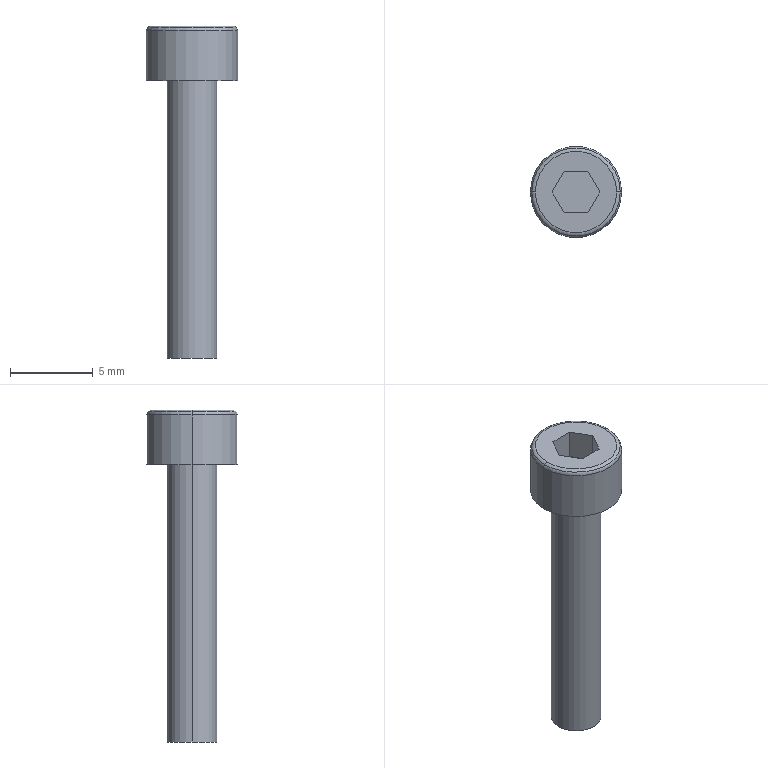Part | Creo | 1 solid | 18 faces | box 5.5 x 5.5 x 20 mm | volume 186.379 mm3 | plane 10 | cylinder 4 | torus 4 | commonest cylinder face diameters 3 x2 5.5 x2
STEP:
#1=CARTESIAN_POINT('',(0.,0.,0.));
#2=DIRECTION('',(0.,0.,1.));
#3=DIRECTION('',(1.,0.,0.));
#4=AXIS2_PLACEMENT_3D('',#1,#2,#3);
#5=CARTESIAN_POINT('',(30.45,156.5,-39.767));
#6=VERTEX_POINT('',#5);
#7=CARTESIAN_POINT('',(33.45,156.5,-39.767));
#8=VERTEX_POINT('',#7);
#9=CARTESIAN_POINT('',(31.95,156.5,-39.767));
#10=DIRECTION('',(0.,0.,-1.));
#11=DIRECTION('',(-1.,0.,0.));
#12=AXIS2_PLACEMENT_3D('',#9,#10,#11);
#13=CIRCLE('',#12,1.5);
#14=EDGE_CURVE('',#6,#8,#13,.T.);
#15=ORIENTED_EDGE('',*,*,#14,.F.);
#16=CARTESIAN_POINT('',(31.95,156.5,-39.767));
#17=DIRECTION('',(0.,0.,-1.));
#18=DIRECTION('',(1.,0.,0.));
#19=AXIS2_PLACEMENT_3D('',#16,#17,#18);
#20=CIRCLE('',#19,1.5);
#21=EDGE_CURVE('',#8,#6,#20,.T.);
#22=ORIENTED_EDGE('',*,*,#21,.F.);
#23=EDGE_LOOP('',(#15,#22));
#24=FACE_OUTER_BOUND('',#23,.F.);
#25=CARTESIAN_POINT('',(31.95,156.5,-39.767));
#26=DIRECTION('',(0.,0.,-1.));
#27=DIRECTION('',(-1.,0.,0.));
#28=AXIS2_PLACEMENT_3D('',#25,#26,#27);
#29=PLANE('',#28);
#30=ADVANCED_FACE('',(#24),#29,.T.);
#31=CARTESIAN_POINT('',(33.45,156.5,-23.067));
#32=VERTEX_POINT('',#31);
#33=CARTESIAN_POINT('',(30.45,156.5,-23.067));
#34=VERTEX_POINT('',#33);
#35=CARTESIAN_POINT('',(31.95,156.5,-23.067));
#36=DIRECTION('',(0.,0.,1.));
#37=DIRECTION('',(1.,0.,0.));
#38=AXIS2_PLACEMENT_3D('',#35,#36,#37);
#39=CIRCLE('',#38,1.5);
#40=EDGE_CURVE('',#32,#34,#39,.T.);
#41=ORIENTED_EDGE('',*,*,#40,.T.);
#42=CARTESIAN_POINT('',(30.45,156.5,-23.067));
#43=DIRECTION('',(0.,0.,-1.));
#44=VECTOR('',#43,16.7);
#45=LINE('',#42,#44);
#46=EDGE_CURVE('',#34,#6,#45,.T.);
#47=ORIENTED_EDGE('',*,*,#46,.T.);
#48=ORIENTED_EDGE('',*,*,#14,.T.);
#49=CARTESIAN_POINT('',(33.45,156.5,-23.067));
#50=DIRECTION('',(0.,0.,-1.));
#51=VECTOR('',#50,16.7);
#52=LINE('',#49,#51);
#53=EDGE_CURVE('',#32,#8,#52,.T.);
#54=ORIENTED_EDGE('',*,*,#53,.F.);
#55=EDGE_LOOP('',(#41,#47,#48,#54));
#56=FACE_OUTER_BOUND('',#55,.F.);
#57=CARTESIAN_POINT('',(31.95,156.5,-19.767));
#58=DIRECTION('',(0.,0.,-1.));
#59=DIRECTION('',(-1.,0.,0.));
#60=AXIS2_PLACEMENT_3D('',#57,#58,#59);
#61=CYLINDRICAL_SURFACE('',#60,1.5);
#62=ADVANCED_FACE('',(#56),#61,.T.);
#63=CARTESIAN_POINT('',(29.2,156.5,-23.067));
#64=VERTEX_POINT('',#63);
#65=CARTESIAN_POINT('',(34.7,156.5,-23.067));
#66=VERTEX_POINT('',#65);
#67=CARTESIAN_POINT('',(31.95,156.5,-23.067));
#68=DIRECTION('',(0.,0.,-1.));
#69=DIRECTION('',(-1.,0.,0.));
#70=AXIS2_PLACEMENT_3D('',#67,#68,#69);
#71=CIRCLE('',#70,2.75);
#72=EDGE_CURVE('',#64,#66,#71,.T.);
#73=ORIENTED_EDGE('',*,*,#72,.F.);
#74=CARTESIAN_POINT('',(31.95,156.5,-23.067));
#75=DIRECTION('',(0.,0.,-1.));
#76=DIRECTION('',(1.,0.,0.));
#77=AXIS2_PLACEMENT_3D('',#74,#75,#76);
#78=CIRCLE('',#77,2.75);
#79=EDGE_CURVE('',#66,#64,#78,.T.);
#80=ORIENTED_EDGE('',*,*,#79,.F.);
#81=EDGE_LOOP('',(#73,#80));
#82=FACE_OUTER_BOUND('',#81,.F.);
#83=CARTESIAN_POINT('',(31.95,156.5,-23.067));
#84=DIRECTION('',(0.,0.,1.));
#85=DIRECTION('',(-1.,0.,0.));
#86=AXIS2_PLACEMENT_3D('',#83,#84,#85);
#87=CIRCLE('',#86,1.5);
#88=EDGE_CURVE('',#34,#32,#87,.T.);
#89=ORIENTED_EDGE('',*,*,#88,.F.);
#90=ORIENTED_EDGE('',*,*,#40,.F.);
#91=EDGE_LOOP('',(#89,#90));
#92=FACE_BOUND('',#91,.F.);
#93=CARTESIAN_POINT('',(31.95,158.,-23.067));
#94=DIRECTION('',(0.,0.,-1.));
#95=DIRECTION('',(-1.,0.,0.));
#96=AXIS2_PLACEMENT_3D('',#93,#94,#95);
#97=PLANE('',#96);
#98=ADVANCED_FACE('',(#82,#92),#97,.T.);
#99=CARTESIAN_POINT('',(34.7,156.5,-20.067));
#100=VERTEX_POINT('',#99);
#101=CARTESIAN_POINT('',(29.2,156.5,-20.067));
#102=VERTEX_POINT('',#101);
#103=CARTESIAN_POINT('',(31.95,156.5,-20.067));
#104=DIRECTION('',(0.,0.,1.));
#105=DIRECTION('',(1.,0.,0.));
#106=AXIS2_PLACEMENT_3D('',#103,#104,#105);
#107=CIRCLE('',#106,2.75);
#108=EDGE_CURVE('',#100,#102,#107,.T.);
#109=ORIENTED_EDGE('',*,*,#108,.T.);
#110=CARTESIAN_POINT('',(29.2,156.5,-20.067));
#111=DIRECTION('',(0.,0.,-1.));
#112=VECTOR('',#111,3.);
#113=LINE('',#110,#112);
#114=EDGE_CURVE('',#102,#64,#113,.T.);
#115=ORIENTED_EDGE('',*,*,#114,.T.);
#116=ORIENTED_EDGE('',*,*,#72,.T.);
#117=CARTESIAN_POINT('',(34.7,156.5,-20.067));
#118=DIRECTION('',(0.,0.,-1.));
#119=VECTOR('',#118,3.);
#120=LINE('',#117,#119);
#121=EDGE_CURVE('',#100,#66,#120,.T.);
#122=ORIENTED_EDGE('',*,*,#121,.F.);
#123=EDGE_LOOP('',(#109,#115,#116,#122));
#124=FACE_OUTER_BOUND('',#123,.F.);
#125=CARTESIAN_POINT('',(31.95,156.5,-19.767));
#126=DIRECTION('',(0.,0.,-1.));
#127=DIRECTION('',(-1.,0.,0.));
#128=AXIS2_PLACEMENT_3D('',#125,#126,#127);
#129=CYLINDRICAL_SURFACE('',#128,2.75);
#130=ADVANCED_FACE('',(#124),#129,.T.);
#131=ORIENTED_EDGE('',*,*,#108,.F.);
#132=CARTESIAN_POINT('',(34.612,156.5,-19.855));
#133=VERTEX_POINT('',#132);
#134=CARTESIAN_POINT('',(34.4,156.5,-20.067));
#135=DIRECTION('',(0.,-1.,0.));
#136=DIRECTION('',(1.,0.,0.));
#137=AXIS2_PLACEMENT_3D('',#134,#135,#136);
#138=CIRCLE('',#137,0.3);
#139=EDGE_CURVE('',#100,#133,#138,.T.);
#140=ORIENTED_EDGE('',*,*,#139,.T.);
#141=CARTESIAN_POINT('',(29.288,156.5,-19.855));
#142=VERTEX_POINT('',#141);
#143=CARTESIAN_POINT('',(31.95,156.5,-19.855));
#144=DIRECTION('',(0.,0.,1.));
#145=DIRECTION('',(1.,0.,0.));
#146=AXIS2_PLACEMENT_3D('',#143,#144,#145);
#147=CIRCLE('',#146,2.662);
#148=EDGE_CURVE('',#133,#142,#147,.T.);
#149=ORIENTED_EDGE('',*,*,#148,.T.);
#150=CARTESIAN_POINT('',(29.5,156.5,-20.067));
#151=DIRECTION('',(0.,1.,0.));
#152=DIRECTION('',(-1.,0.,0.));
#153=AXIS2_PLACEMENT_3D('',#150,#151,#152);
#154=CIRCLE('',#153,0.3);
#155=EDGE_CURVE('',#102,#142,#154,.T.);
#156=ORIENTED_EDGE('',*,*,#155,.F.);
#157=EDGE_LOOP('',(#131,#140,#149,#156));
#158=FACE_OUTER_BOUND('',#157,.F.);
#159=CARTESIAN_POINT('',(31.95,156.5,-20.067));
#160=DIRECTION('',(0.,0.,1.));
#161=DIRECTION('',(1.,0.,0.));
#162=AXIS2_PLACEMENT_3D('',#159,#160,#161);
#163=TOROIDAL_SURFACE('',#162,2.45,0.3);
#164=ADVANCED_FACE('',(#158),#163,.T.);
#165=CARTESIAN_POINT('',(31.95,156.5,-20.067));
#166=DIRECTION('',(0.,0.,1.));
#167=DIRECTION('',(-1.,0.,0.));
#168=AXIS2_PLACEMENT_3D('',#165,#166,#167);
#169=CIRCLE('',#168,2.75);
#170=EDGE_CURVE('',#102,#100,#169,.T.);
#171=ORIENTED_EDGE('',*,*,#170,.F.);
#172=ORIENTED_EDGE('',*,*,#155,.T.);
#173=CARTESIAN_POINT('',(31.95,156.5,-19.855));
#174=DIRECTION('',(0.,0.,1.));
#175=DIRECTION('',(-1.,0.,0.));
#176=AXIS2_PLACEMENT_3D('',#173,#174,#175);
#177=CIRCLE('',#176,2.662);
#178=EDGE_CURVE('',#142,#133,#177,.T.);
#179=ORIENTED_EDGE('',*,*,#178,.T.);
#180=ORIENTED_EDGE('',*,*,#139,.F.);
#181=EDGE_LOOP('',(#171,#172,#179,#180));
#182=FACE_OUTER_BOUND('',#181,.F.);
#183=CARTESIAN_POINT('',(31.95,156.5,-20.067));
#184=DIRECTION('',(0.,0.,1.));
#185=DIRECTION('',(1.,0.,0.));
#186=AXIS2_PLACEMENT_3D('',#183,#184,#185);
#187=TOROIDAL_SURFACE('',#186,2.45,0.3);
#188=ADVANCED_FACE('',(#182),#187,.T.);
#189=ORIENTED_EDGE('',*,*,#170,.T.);
#190=ORIENTED_EDGE('',*,*,#121,.T.);
#191=ORIENTED_EDGE('',*,*,#79,.T.);
#192=ORIENTED_EDGE('',*,*,#114,.F.);
#193=EDGE_LOOP('',(#189,#190,#191,#192));
#194=FACE_OUTER_BOUND('',#193,.F.);
#195=CARTESIAN_POINT('',(31.95,156.5,-19.767));
#196=DIRECTION('',(0.,0.,-1.));
#197=DIRECTION('',(-1.,0.,0.));
#198=AXIS2_PLACEMENT_3D('',#195,#196,#197);
#199=CYLINDRICAL_SURFACE('',#198,2.75);
#200=ADVANCED_FACE('',(#194),#199,.T.);
#201=CARTESIAN_POINT('',(29.5,156.5,-19.767));
#202=VERTEX_POINT('',#201);
#203=CARTESIAN_POINT('',(34.4,156.5,-19.767));
#204=VERTEX_POINT('',#203);
#205=CARTESIAN_POINT('',(31.95,156.5,-19.767));
#206=DIRECTION('',(0.,0.,1.));
#207=DIRECTION('',(-1.,0.,0.));
#208=AXIS2_PLACEMENT_3D('',#205,#206,#207);
#209=CIRCLE('',#208,2.45);
#210=EDGE_CURVE('',#202,#204,#209,.T.);
#211=ORIENTED_EDGE('',*,*,#210,.T.);
#212=CARTESIAN_POINT('',(34.4,156.5,-20.067));
#213=DIRECTION('',(0.,-1.,0.));
#214=DIRECTION('',(0.7071,0.,0.7071));
#215=AXIS2_PLACEMENT_3D('',#212,#213,#214);
#216=CIRCLE('',#215,0.3);
#217=EDGE_CURVE('',#133,#204,#216,.T.);
#218=ORIENTED_EDGE('',*,*,#217,.F.);
#219=ORIENTED_EDGE('',*,*,#178,.F.);
#220=CARTESIAN_POINT('',(29.5,156.5,-20.067));
#221=DIRECTION('',(0.,1.,0.));
#222=DIRECTION('',(-0.7071,0.,0.7071));
#223=AXIS2_PLACEMENT_3D('',#220,#221,#222);
#224=CIRCLE('',#223,0.3);
#225=EDGE_CURVE('',#142,#202,#224,.T.);
#226=ORIENTED_EDGE('',*,*,#225,.T.);
#227=EDGE_LOOP('',(#211,#218,#219,#226));
#228=FACE_OUTER_BOUND('',#227,.F.);
#229=CARTESIAN_POINT('',(31.95,156.5,-20.067));
#230=DIRECTION('',(0.,0.,1.));
#231=DIRECTION('',(1.,0.,0.));
#232=AXIS2_PLACEMENT_3D('',#229,#230,#231);
#233=TOROIDAL_SURFACE('',#232,2.45,0.3);
#234=ADVANCED_FACE('',(#228),#233,.T.);
#235=CARTESIAN_POINT('',(31.95,156.5,-19.767));
#236=DIRECTION('',(0.,0.,1.));
#237=DIRECTION('',(1.,0.,0.));
#238=AXIS2_PLACEMENT_3D('',#235,#236,#237);
#239=CIRCLE('',#238,2.45);
#240=EDGE_CURVE('',#204,#202,#239,.T.);
#241=ORIENTED_EDGE('',*,*,#240,.F.);
#242=ORIENTED_EDGE('',*,*,#210,.F.);
#243=EDGE_LOOP('',(#241,#242));
#244=FACE_OUTER_BOUND('',#243,.F.);
#245=CARTESIAN_POINT('',(31.228,155.25,-19.767));
#246=VERTEX_POINT('',#245);
#247=CARTESIAN_POINT('',(30.507,156.5,-19.767));
#248=VERTEX_POINT('',#247);
#249=CARTESIAN_POINT('',(31.228,155.25,-19.767));
#250=DIRECTION('',(-0.5,0.866,0.));
#251=VECTOR('',#250,1.443);
#252=LINE('',#249,#251);
#253=EDGE_CURVE('',#246,#248,#252,.T.);
#254=ORIENTED_EDGE('',*,*,#253,.F.);
#255=CARTESIAN_POINT('',(32.672,155.25,-19.767));
#256=VERTEX_POINT('',#255);
#257=CARTESIAN_POINT('',(32.672,155.25,-19.767));
#258=DIRECTION('',(-1.,0.,0.));
#259=VECTOR('',#258,1.443);
#260=LINE('',#257,#259);
#261=EDGE_CURVE('',#256,#246,#260,.T.);
#262=ORIENTED_EDGE('',*,*,#261,.F.);
#263=CARTESIAN_POINT('',(33.393,156.5,-19.767));
#264=VERTEX_POINT('',#263);
#265=CARTESIAN_POINT('',(33.393,156.5,-19.767));
#266=DIRECTION('',(-0.5,-0.866,0.));
#267=VECTOR('',#266,1.443);
#268=LINE('',#265,#267);
#269=EDGE_CURVE('',#264,#256,#268,.T.);
#270=ORIENTED_EDGE('',*,*,#269,.F.);
#271=CARTESIAN_POINT('',(32.672,157.75,-19.767));
#272=VERTEX_POINT('',#271);
#273=CARTESIAN_POINT('',(32.672,157.75,-19.767));
#274=DIRECTION('',(0.5,-0.866,0.));
#275=VECTOR('',#274,1.443);
#276=LINE('',#273,#275);
#277=EDGE_CURVE('',#272,#264,#276,.T.);
#278=ORIENTED_EDGE('',*,*,#277,.F.);
#279=CARTESIAN_POINT('',(31.228,157.75,-19.767));
#280=VERTEX_POINT('',#279);
#281=CARTESIAN_POINT('',(31.228,157.75,-19.767));
#282=DIRECTION('',(1.,0.,0.));
#283=VECTOR('',#282,1.443);
#284=LINE('',#281,#283);
#285=EDGE_CURVE('',#280,#272,#284,.T.);
#286=ORIENTED_EDGE('',*,*,#285,.F.);
#287=CARTESIAN_POINT('',(30.507,156.5,-19.767));
#288=DIRECTION('',(0.5,0.866,0.));
#289=VECTOR('',#288,1.443);
#290=LINE('',#287,#289);
#291=EDGE_CURVE('',#248,#280,#290,.T.);
#292=ORIENTED_EDGE('',*,*,#291,.F.);
#293=EDGE_LOOP('',(#254,#262,#270,#278,#286,#292));
#294=FACE_BOUND('',#293,.F.);
#295=CARTESIAN_POINT('',(31.95,159.25,-19.767));
#296=DIRECTION('',(0.,0.,1.));
#297=DIRECTION('',(1.,0.,0.));
#298=AXIS2_PLACEMENT_3D('',#295,#296,#297);
#299=PLANE('',#298);
#300=ADVANCED_FACE('',(#244,#294),#299,.T.);
#301=ORIENTED_EDGE('',*,*,#240,.T.);
#302=ORIENTED_EDGE('',*,*,#225,.F.);
#303=ORIENTED_EDGE('',*,*,#148,.F.);
#304=ORIENTED_EDGE('',*,*,#217,.T.);
#305=EDGE_LOOP('',(#301,#302,#303,#304));
#306=FACE_OUTER_BOUND('',#305,.F.);
#307=CARTESIAN_POINT('',(31.95,156.5,-20.067));
#308=DIRECTION('',(0.,0.,1.));
#309=DIRECTION('',(1.,0.,0.));
#310=AXIS2_PLACEMENT_3D('',#307,#308,#309);
#311=TOROIDAL_SURFACE('',#310,2.45,0.3);
#312=ADVANCED_FACE('',(#306),#311,.T.);
#313=ORIENTED_EDGE('',*,*,#253,.T.);
#314=CARTESIAN_POINT('',(30.507,156.5,-21.567));
#315=VERTEX_POINT('',#314);
#316=CARTESIAN_POINT('',(30.507,156.5,-21.567));
#317=DIRECTION('',(0.,0.,1.));
#318=VECTOR('',#317,1.8);
#319=LINE('',#316,#318);
#320=EDGE_CURVE('',#315,#248,#319,.T.);
#321=ORIENTED_EDGE('',*,*,#320,.F.);
#322=CARTESIAN_POINT('',(31.228,155.25,-21.567));
#323=VERTEX_POINT('',#322);
#324=CARTESIAN_POINT('',(30.507,156.5,-21.567));
#325=DIRECTION('',(0.5,-0.866,0.));
#326=VECTOR('',#325,1.443);
#327=LINE('',#324,#326);
#328=EDGE_CURVE('',#315,#323,#327,.T.);
#329=ORIENTED_EDGE('',*,*,#328,.T.);
#330=CARTESIAN_POINT('',(31.228,155.25,-21.567));
#331=DIRECTION('',(0.,0.,1.));
#332=VECTOR('',#331,1.8);
#333=LINE('',#330,#332);
#334=EDGE_CURVE('',#323,#246,#333,.T.);
#335=ORIENTED_EDGE('',*,*,#334,.T.);
#336=EDGE_LOOP('',(#313,#321,#329,#335));
#337=FACE_OUTER_BOUND('',#336,.F.);
#338=CARTESIAN_POINT('',(30.507,156.5,-21.567));
#339=DIRECTION('',(-0.866,-0.5,0.));
#340=DIRECTION('',(0.5,-0.866,0.));
#341=AXIS2_PLACEMENT_3D('',#338,#339,#340);
#342=PLANE('',#341);
#343=ADVANCED_FACE('',(#337),#342,.F.);
#344=ORIENTED_EDGE('',*,*,#291,.T.);
#345=CARTESIAN_POINT('',(31.228,157.75,-21.567));
#346=VERTEX_POINT('',#345);
#347=CARTESIAN_POINT('',(31.228,157.75,-21.567));
#348=DIRECTION('',(0.,0.,1.));
#349=VECTOR('',#348,1.8);
#350=LINE('',#347,#349);
#351=EDGE_CURVE('',#346,#280,#350,.T.);
#352=ORIENTED_EDGE('',*,*,#351,.F.);
#353=CARTESIAN_POINT('',(31.228,157.75,-21.567));
#354=DIRECTION('',(-0.5,-0.866,0.));
#355=VECTOR('',#354,1.443);
#356=LINE('',#353,#355);
#357=EDGE_CURVE('',#346,#315,#356,.T.);
#358=ORIENTED_EDGE('',*,*,#357,.T.);
#359=ORIENTED_EDGE('',*,*,#320,.T.);
#360=EDGE_LOOP('',(#344,#352,#358,#359));
#361=FACE_OUTER_BOUND('',#360,.F.);
#362=CARTESIAN_POINT('',(31.228,157.75,-21.567));
#363=DIRECTION('',(-0.866,0.5,0.));
#364=DIRECTION('',(-0.5,-0.866,0.));
#365=AXIS2_PLACEMENT_3D('',#362,#363,#364);
#366=PLANE('',#365);
#367=ADVANCED_FACE('',(#361),#366,.F.);
#368=ORIENTED_EDGE('',*,*,#285,.T.);
#369=CARTESIAN_POINT('',(32.672,157.75,-21.567));
#370=VERTEX_POINT('',#369);
#371=CARTESIAN_POINT('',(32.672,157.75,-21.567));
#372=DIRECTION('',(0.,0.,1.));
#373=VECTOR('',#372,1.8);
#374=LINE('',#371,#373);
#375=EDGE_CURVE('',#370,#272,#374,.T.);
#376=ORIENTED_EDGE('',*,*,#375,.F.);
#377=CARTESIAN_POINT('',(32.672,157.75,-21.567));
#378=DIRECTION('',(-1.,0.,0.));
#379=VECTOR('',#378,1.443);
#380=LINE('',#377,#379);
#381=EDGE_CURVE('',#370,#346,#380,.T.);
#382=ORIENTED_EDGE('',*,*,#381,.T.);
#383=ORIENTED_EDGE('',*,*,#351,.T.);
#384=EDGE_LOOP('',(#368,#376,#382,#383));
#385=FACE_OUTER_BOUND('',#384,.F.);
#386=CARTESIAN_POINT('',(32.672,157.75,-21.567));
#387=DIRECTION('',(0.,1.,0.));
#388=DIRECTION('',(-1.,0.,0.));
#389=AXIS2_PLACEMENT_3D('',#386,#387,#388);
#390=PLANE('',#389);
#391=ADVANCED_FACE('',(#385),#390,.F.);
#392=ORIENTED_EDGE('',*,*,#277,.T.);
#393=CARTESIAN_POINT('',(33.393,156.5,-21.567));
#394=VERTEX_POINT('',#393);
#395=CARTESIAN_POINT('',(33.393,156.5,-21.567));
#396=DIRECTION('',(0.,0.,1.));
#397=VECTOR('',#396,1.8);
#398=LINE('',#395,#397);
#399=EDGE_CURVE('',#394,#264,#398,.T.);
#400=ORIENTED_EDGE('',*,*,#399,.F.);
#401=CARTESIAN_POINT('',(33.393,156.5,-21.567));
#402=DIRECTION('',(-0.5,0.866,0.));
#403=VECTOR('',#402,1.443);
#404=LINE('',#401,#403);
#405=EDGE_CURVE('',#394,#370,#404,.T.);
#406=ORIENTED_EDGE('',*,*,#405,.T.);
#407=ORIENTED_EDGE('',*,*,#375,.T.);
#408=EDGE_LOOP('',(#392,#400,#406,#407));
#409=FACE_OUTER_BOUND('',#408,.F.);
#410=CARTESIAN_POINT('',(33.393,156.5,-21.567));
#411=DIRECTION('',(0.866,0.5,0.));
#412=DIRECTION('',(-0.5,0.866,0.));
#413=AXIS2_PLACEMENT_3D('',#410,#411,#412);
#414=PLANE('',#413);
#415=ADVANCED_FACE('',(#409),#414,.F.);
#416=ORIENTED_EDGE('',*,*,#269,.T.);
#417=CARTESIAN_POINT('',(32.672,155.25,-21.567));
#418=VERTEX_POINT('',#417);
#419=CARTESIAN_POINT('',(32.672,155.25,-21.567));
#420=DIRECTION('',(0.,0.,1.));
#421=VECTOR('',#420,1.8);
#422=LINE('',#419,#421);
#423=EDGE_CURVE('',#418,#256,#422,.T.);
#424=ORIENTED_EDGE('',*,*,#423,.F.);
#425=CARTESIAN_POINT('',(32.672,155.25,-21.567));
#426=DIRECTION('',(0.5,0.866,0.));
#427=VECTOR('',#426,1.443);
#428=LINE('',#425,#427);
#429=EDGE_CURVE('',#418,#394,#428,.T.);
#430=ORIENTED_EDGE('',*,*,#429,.T.);
#431=ORIENTED_EDGE('',*,*,#399,.T.);
#432=EDGE_LOOP('',(#416,#424,#430,#431));
#433=FACE_OUTER_BOUND('',#432,.F.);
#434=CARTESIAN_POINT('',(32.672,155.25,-21.567));
#435=DIRECTION('',(0.866,-0.5,0.));
#436=DIRECTION('',(0.5,0.866,0.));
#437=AXIS2_PLACEMENT_3D('',#434,#435,#436);
#438=PLANE('',#437);
#439=ADVANCED_FACE('',(#433),#438,.F.);
#440=ORIENTED_EDGE('',*,*,#261,.T.);
#441=ORIENTED_EDGE('',*,*,#334,.F.);
#442=CARTESIAN_POINT('',(31.228,155.25,-21.567));
#443=DIRECTION('',(1.,0.,0.));
#444=VECTOR('',#443,1.443);
#445=LINE('',#442,#444);
#446=EDGE_CURVE('',#323,#418,#445,.T.);
#447=ORIENTED_EDGE('',*,*,#446,.T.);
#448=ORIENTED_EDGE('',*,*,#423,.T.);
#449=EDGE_LOOP('',(#440,#441,#447,#448));
#450=FACE_OUTER_BOUND('',#449,.F.);
#451=CARTESIAN_POINT('',(31.228,155.25,-21.567));
#452=DIRECTION('',(0.,-1.,0.));
#453=DIRECTION('',(0.,0.,-1.));
#454=AXIS2_PLACEMENT_3D('',#451,#452,#453);
#455=PLANE('',#454);
#456=ADVANCED_FACE('',(#450),#455,.F.);
#457=ORIENTED_EDGE('',*,*,#328,.F.);
#458=ORIENTED_EDGE('',*,*,#357,.F.);
#459=ORIENTED_EDGE('',*,*,#381,.F.);
#460=ORIENTED_EDGE('',*,*,#405,.F.);
#461=ORIENTED_EDGE('',*,*,#429,.F.);
#462=ORIENTED_EDGE('',*,*,#446,.F.);
#463=EDGE_LOOP('',(#457,#458,#459,#460,#461,#462));
#464=FACE_OUTER_BOUND('',#463,.F.);
#465=CARTESIAN_POINT('',(31.95,161.5,-21.567));
#466=DIRECTION('',(0.,0.,1.));
#467=DIRECTION('',(1.,0.,0.));
#468=AXIS2_PLACEMENT_3D('',#465,#466,#467);
#469=PLANE('',#468);
#470=ADVANCED_FACE('',(#464),#469,.T.);
#471=ORIENTED_EDGE('',*,*,#88,.T.);
#472=ORIENTED_EDGE('',*,*,#53,.T.);
#473=ORIENTED_EDGE('',*,*,#21,.T.);
#474=ORIENTED_EDGE('',*,*,#46,.F.);
#475=EDGE_LOOP('',(#471,#472,#473,#474));
#476=FACE_OUTER_BOUND('',#475,.F.);
#477=CARTESIAN_POINT('',(31.95,156.5,-19.767));
#478=DIRECTION('',(0.,0.,-1.));
#479=DIRECTION('',(-1.,0.,0.));
#480=AXIS2_PLACEMENT_3D('',#477,#478,#479);
#481=CYLINDRICAL_SURFACE('',#480,1.5);
#482=ADVANCED_FACE('',(#476),#481,.T.);
#483=CLOSED_SHELL('',(#30,#62,#98,#130,#164,#188,#200,#234,#300,#312,#343,#367,#391,#415,#439,#456,#470,#482));
#484=MANIFOLD_SOLID_BREP('',#483);
#485=(LENGTH_UNIT()NAMED_UNIT(*)SI_UNIT(.MILLI.,.METRE.));
#486=UNCERTAINTY_MEASURE_WITH_UNIT(LENGTH_MEASURE(0.002146),#485,'','');
#487=(NAMED_UNIT(*)PLANE_ANGLE_UNIT()SI_UNIT($,.RADIAN.));
#488=PLANE_ANGLE_MEASURE_WITH_UNIT(PLANE_ANGLE_MEASURE(0.01745),#487);
#489=(CONVERSION_BASED_UNIT('DEGREE',#488)NAMED_UNIT(*)PLANE_ANGLE_UNIT());
#490=(NAMED_UNIT(*)SI_UNIT($,.STERADIAN.)SOLID_ANGLE_UNIT());
#491=(GEOMETRIC_REPRESENTATION_CONTEXT(3)GLOBAL_UNCERTAINTY_ASSIGNED_CONTEXT((#486))GLOBAL_UNIT_ASSIGNED_CONTEXT((#485,#489,#490))REPRESENTATION_CONTEXT('',''));
#492=ADVANCED_BREP_SHAPE_REPRESENTATION('',(#4,#484),#491);